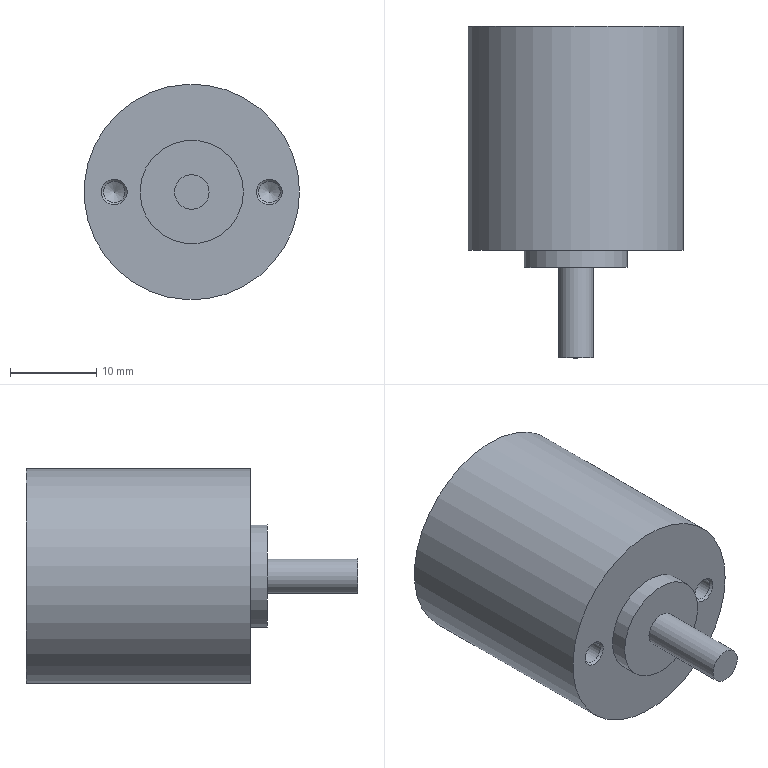Part | NX | features DATUM_CSYS 5, SKETCH 4, EXTRUDE 3, SIMPLE HOLE 2, SYMBOLIC_THREAD 2, HOLE PACKAGE 1 | 1 solid | 13 faces | box 25 x 38.5 x 25 mm | volume 13059 mm3 | cylinder 5 | plane 4 | cone 4 | commonest cylinder face diameters 2.5 x2 4 x1 12 x1 25 x1
STEP:
#1=CARTESIAN_POINT('',(12.5,-26.,0.));
#2=VERTEX_POINT('',#1);
#3=CARTESIAN_POINT('',(0.,-26.,0.));
#4=DIRECTION('',(0.,-1.,0.));
#5=DIRECTION('',(1.,0.,0.));
#6=AXIS2_PLACEMENT_3D('',#3,#4,#5);
#7=CIRCLE('',#6,12.5);
#8=EDGE_CURVE('',#2,#2,#7,.T.);
#9=ORIENTED_EDGE('',*,*,#8,.F.);
#10=EDGE_LOOP('',(#9));
#11=FACE_BOUND('',#10,.T.);
#12=CARTESIAN_POINT('',(12.5,0.,0.));
#13=VERTEX_POINT('',#12);
#14=CARTESIAN_POINT('',(0.,0.,0.));
#15=DIRECTION('',(0.,-1.,0.));
#16=DIRECTION('',(1.,0.,0.));
#17=AXIS2_PLACEMENT_3D('',#14,#15,#16);
#18=CIRCLE('',#17,12.5);
#19=EDGE_CURVE('',#13,#13,#18,.T.);
#20=ORIENTED_EDGE('',*,*,#19,.T.);
#21=EDGE_LOOP('',(#20));
#22=FACE_BOUND('',#21,.T.);
#23=CARTESIAN_POINT('',(0.,-26.,0.));
#24=DIRECTION('',(0.,1.,0.));
#25=DIRECTION('',(0.,0.,1.));
#26=AXIS2_PLACEMENT_3D('',#23,#24,#25);
#27=CYLINDRICAL_SURFACE('',#26,12.5);
#28=ADVANCED_FACE('',(#11,#22),#27,.T.);
#29=CARTESIAN_POINT('',(9.,-26.,-1.5));
#30=VERTEX_POINT('',#29);
#31=CARTESIAN_POINT('',(9.,-26.,0.));
#32=DIRECTION('',(0.,-1.,0.));
#33=DIRECTION('',(0.,0.,-1.));
#34=AXIS2_PLACEMENT_3D('',#31,#32,#33);
#35=CIRCLE('',#34,1.5);
#36=EDGE_CURVE('',#30,#30,#35,.F.);
#37=ORIENTED_EDGE('',*,*,#36,.T.);
#38=EDGE_LOOP('',(#37));
#39=FACE_BOUND('',#38,.T.);
#40=CARTESIAN_POINT('',(-9.,-26.,-1.5));
#41=VERTEX_POINT('',#40);
#42=CARTESIAN_POINT('',(-9.,-26.,0.));
#43=DIRECTION('',(0.,-1.,0.));
#44=DIRECTION('',(0.,0.,-1.));
#45=AXIS2_PLACEMENT_3D('',#42,#43,#44);
#46=CIRCLE('',#45,1.5);
#47=EDGE_CURVE('',#41,#41,#46,.F.);
#48=ORIENTED_EDGE('',*,*,#47,.T.);
#49=EDGE_LOOP('',(#48));
#50=FACE_BOUND('',#49,.T.);
#51=CARTESIAN_POINT('',(6.,-26.,0.));
#52=VERTEX_POINT('',#51);
#53=CARTESIAN_POINT('',(0.,-26.,0.));
#54=DIRECTION('',(0.,-1.,0.));
#55=DIRECTION('',(1.,0.,0.));
#56=AXIS2_PLACEMENT_3D('',#53,#54,#55);
#57=CIRCLE('',#56,6.);
#58=EDGE_CURVE('',#52,#52,#57,.T.);
#59=ORIENTED_EDGE('',*,*,#58,.F.);
#60=EDGE_LOOP('',(#59));
#61=FACE_BOUND('',#60,.T.);
#62=ORIENTED_EDGE('',*,*,#8,.T.);
#63=EDGE_LOOP('',(#62));
#64=FACE_BOUND('',#63,.T.);
#65=CARTESIAN_POINT('',(0.,-26.,0.));
#66=DIRECTION('',(0.,-1.,0.));
#67=DIRECTION('',(0.,0.,-1.));
#68=AXIS2_PLACEMENT_3D('',#65,#66,#67);
#69=PLANE('',#68);
#70=ADVANCED_FACE('',(#39,#50,#61,#64),#69,.T.);
#71=ORIENTED_EDGE('',*,*,#19,.F.);
#72=EDGE_LOOP('',(#71));
#73=FACE_BOUND('',#72,.T.);
#74=CARTESIAN_POINT('',(0.,0.,0.));
#75=DIRECTION('',(0.,-1.,0.));
#76=DIRECTION('',(0.,0.,-1.));
#77=AXIS2_PLACEMENT_3D('',#74,#75,#76);
#78=PLANE('',#77);
#79=ADVANCED_FACE('',(#73),#78,.F.);
#80=CARTESIAN_POINT('',(6.,-28.,0.));
#81=VERTEX_POINT('',#80);
#82=CARTESIAN_POINT('',(0.,-28.,0.));
#83=DIRECTION('',(0.,-1.,0.));
#84=DIRECTION('',(1.,0.,0.));
#85=AXIS2_PLACEMENT_3D('',#82,#83,#84);
#86=CIRCLE('',#85,6.);
#87=EDGE_CURVE('',#81,#81,#86,.T.);
#88=ORIENTED_EDGE('',*,*,#87,.F.);
#89=EDGE_LOOP('',(#88));
#90=FACE_BOUND('',#89,.T.);
#91=ORIENTED_EDGE('',*,*,#58,.T.);
#92=EDGE_LOOP('',(#91));
#93=FACE_BOUND('',#92,.T.);
#94=CARTESIAN_POINT('',(0.,-28.,0.));
#95=DIRECTION('',(0.,1.,0.));
#96=DIRECTION('',(0.,0.,1.));
#97=AXIS2_PLACEMENT_3D('',#94,#95,#96);
#98=CYLINDRICAL_SURFACE('',#97,6.);
#99=ADVANCED_FACE('',(#90,#93),#98,.T.);
#100=CARTESIAN_POINT('',(2.,-28.,0.));
#101=VERTEX_POINT('',#100);
#102=CARTESIAN_POINT('',(0.,-28.,0.));
#103=DIRECTION('',(0.,-1.,0.));
#104=DIRECTION('',(1.,0.,0.));
#105=AXIS2_PLACEMENT_3D('',#102,#103,#104);
#106=CIRCLE('',#105,2.);
#107=EDGE_CURVE('',#101,#101,#106,.T.);
#108=ORIENTED_EDGE('',*,*,#107,.F.);
#109=EDGE_LOOP('',(#108));
#110=FACE_BOUND('',#109,.T.);
#111=ORIENTED_EDGE('',*,*,#87,.T.);
#112=EDGE_LOOP('',(#111));
#113=FACE_BOUND('',#112,.T.);
#114=CARTESIAN_POINT('',(0.,-28.,0.));
#115=DIRECTION('',(0.,-1.,0.));
#116=DIRECTION('',(0.,0.,-1.));
#117=AXIS2_PLACEMENT_3D('',#114,#115,#116);
#118=PLANE('',#117);
#119=ADVANCED_FACE('',(#110,#113),#118,.T.);
#120=CARTESIAN_POINT('',(2.,-38.5,0.));
#121=VERTEX_POINT('',#120);
#122=CARTESIAN_POINT('',(0.,-38.5,0.));
#123=DIRECTION('',(0.,-1.,0.));
#124=DIRECTION('',(1.,0.,0.));
#125=AXIS2_PLACEMENT_3D('',#122,#123,#124);
#126=CIRCLE('',#125,2.);
#127=EDGE_CURVE('',#121,#121,#126,.T.);
#128=ORIENTED_EDGE('',*,*,#127,.F.);
#129=EDGE_LOOP('',(#128));
#130=FACE_BOUND('',#129,.T.);
#131=ORIENTED_EDGE('',*,*,#107,.T.);
#132=EDGE_LOOP('',(#131));
#133=FACE_BOUND('',#132,.T.);
#134=CARTESIAN_POINT('',(0.,-38.5,0.));
#135=DIRECTION('',(0.,1.,0.));
#136=DIRECTION('',(0.,0.,1.));
#137=AXIS2_PLACEMENT_3D('',#134,#135,#136);
#138=CYLINDRICAL_SURFACE('',#137,2.);
#139=ADVANCED_FACE('',(#130,#133),#138,.T.);
#140=ORIENTED_EDGE('',*,*,#127,.T.);
#141=EDGE_LOOP('',(#140));
#142=FACE_BOUND('',#141,.T.);
#143=CARTESIAN_POINT('',(0.,-38.5,0.));
#144=DIRECTION('',(0.,-1.,0.));
#145=DIRECTION('',(0.,0.,-1.));
#146=AXIS2_PLACEMENT_3D('',#143,#144,#145);
#147=PLANE('',#146);
#148=ADVANCED_FACE('',(#142),#147,.T.);
#149=CARTESIAN_POINT('',(-9.,-20.,1.25));
#150=VERTEX_POINT('',#149);
#151=CARTESIAN_POINT('',(-9.,-20.,0.));
#152=DIRECTION('',(0.,1.,0.));
#153=DIRECTION('',(0.,0.,1.));
#154=AXIS2_PLACEMENT_3D('',#151,#152,#153);
#155=CIRCLE('',#154,1.25);
#156=EDGE_CURVE('',#150,#150,#155,.F.);
#157=ORIENTED_EDGE('',*,*,#156,.T.);
#158=EDGE_LOOP('',(#157));
#159=FACE_BOUND('',#158,.T.);
#160=CARTESIAN_POINT('',(-9.,-19.249,0.));
#161=VERTEX_POINT('',#160);
#162=VERTEX_LOOP('',#161);
#163=FACE_BOUND('',#162,.T.);
#164=CARTESIAN_POINT('',(-9.,-20.,0.));
#165=DIRECTION('',(0.,-1.,0.));
#166=DIRECTION('',(0.,0.,-1.));
#167=AXIS2_PLACEMENT_3D('',#164,#165,#166);
#168=CONICAL_SURFACE('',#167,1.25,1.03);
#169=ADVANCED_FACE('',(#159,#163),#168,.F.);
#170=CARTESIAN_POINT('',(-9.,-25.75,-1.25));
#171=VERTEX_POINT('',#170);
#172=CARTESIAN_POINT('',(-9.,-25.75,0.));
#173=DIRECTION('',(0.,-1.,0.));
#174=DIRECTION('',(0.,0.,-1.));
#175=AXIS2_PLACEMENT_3D('',#172,#173,#174);
#176=CIRCLE('',#175,1.25);
#177=EDGE_CURVE('',#171,#171,#176,.T.);
#178=ORIENTED_EDGE('',*,*,#177,.T.);
#179=EDGE_LOOP('',(#178));
#180=FACE_BOUND('',#179,.T.);
#181=ORIENTED_EDGE('',*,*,#156,.F.);
#182=EDGE_LOOP('',(#181));
#183=FACE_BOUND('',#182,.T.);
#184=CARTESIAN_POINT('',(-9.,-26.,0.));
#185=DIRECTION('',(0.,1.,0.));
#186=DIRECTION('',(0.,0.,1.));
#187=AXIS2_PLACEMENT_3D('',#184,#185,#186);
#188=CYLINDRICAL_SURFACE('',#187,1.25);
#189=ADVANCED_FACE('',(#180,#183),#188,.F.);
#190=ORIENTED_EDGE('',*,*,#177,.F.);
#191=EDGE_LOOP('',(#190));
#192=FACE_BOUND('',#191,.T.);
#193=ORIENTED_EDGE('',*,*,#47,.F.);
#194=EDGE_LOOP('',(#193));
#195=FACE_BOUND('',#194,.T.);
#196=CARTESIAN_POINT('',(-9.,-26.,0.));
#197=DIRECTION('',(0.,-1.,0.));
#198=DIRECTION('',(0.,0.,-1.));
#199=AXIS2_PLACEMENT_3D('',#196,#197,#198);
#200=CONICAL_SURFACE('',#199,1.5,0.7854);
#201=ADVANCED_FACE('',(#192,#195),#200,.F.);
#202=CARTESIAN_POINT('',(9.,-20.,1.25));
#203=VERTEX_POINT('',#202);
#204=CARTESIAN_POINT('',(9.,-20.,0.));
#205=DIRECTION('',(0.,1.,0.));
#206=DIRECTION('',(0.,0.,1.));
#207=AXIS2_PLACEMENT_3D('',#204,#205,#206);
#208=CIRCLE('',#207,1.25);
#209=EDGE_CURVE('',#203,#203,#208,.F.);
#210=ORIENTED_EDGE('',*,*,#209,.T.);
#211=EDGE_LOOP('',(#210));
#212=FACE_BOUND('',#211,.T.);
#213=CARTESIAN_POINT('',(9.,-19.249,0.));
#214=VERTEX_POINT('',#213);
#215=VERTEX_LOOP('',#214);
#216=FACE_BOUND('',#215,.T.);
#217=CARTESIAN_POINT('',(9.,-20.,0.));
#218=DIRECTION('',(0.,-1.,0.));
#219=DIRECTION('',(0.,0.,-1.));
#220=AXIS2_PLACEMENT_3D('',#217,#218,#219);
#221=CONICAL_SURFACE('',#220,1.25,1.03);
#222=ADVANCED_FACE('',(#212,#216),#221,.F.);
#223=CARTESIAN_POINT('',(9.,-25.75,-1.25));
#224=VERTEX_POINT('',#223);
#225=CARTESIAN_POINT('',(9.,-25.75,0.));
#226=DIRECTION('',(0.,-1.,0.));
#227=DIRECTION('',(0.,0.,-1.));
#228=AXIS2_PLACEMENT_3D('',#225,#226,#227);
#229=CIRCLE('',#228,1.25);
#230=EDGE_CURVE('',#224,#224,#229,.T.);
#231=ORIENTED_EDGE('',*,*,#230,.T.);
#232=EDGE_LOOP('',(#231));
#233=FACE_BOUND('',#232,.T.);
#234=ORIENTED_EDGE('',*,*,#209,.F.);
#235=EDGE_LOOP('',(#234));
#236=FACE_BOUND('',#235,.T.);
#237=CARTESIAN_POINT('',(9.,-26.,0.));
#238=DIRECTION('',(0.,1.,0.));
#239=DIRECTION('',(0.,0.,1.));
#240=AXIS2_PLACEMENT_3D('',#237,#238,#239);
#241=CYLINDRICAL_SURFACE('',#240,1.25);
#242=ADVANCED_FACE('',(#233,#236),#241,.F.);
#243=ORIENTED_EDGE('',*,*,#230,.F.);
#244=EDGE_LOOP('',(#243));
#245=FACE_BOUND('',#244,.T.);
#246=ORIENTED_EDGE('',*,*,#36,.F.);
#247=EDGE_LOOP('',(#246));
#248=FACE_BOUND('',#247,.T.);
#249=CARTESIAN_POINT('',(9.,-26.,0.));
#250=DIRECTION('',(0.,-1.,0.));
#251=DIRECTION('',(0.,0.,-1.));
#252=AXIS2_PLACEMENT_3D('',#249,#250,#251);
#253=CONICAL_SURFACE('',#252,1.5,0.7854);
#254=ADVANCED_FACE('',(#245,#248),#253,.F.);
#255=CLOSED_SHELL('',(#28,#70,#79,#99,#119,#139,#148,#169,#189,#201,#222,#242,#254));
#256=MANIFOLD_SOLID_BREP('',#255);
#257=(LENGTH_UNIT()NAMED_UNIT(*)SI_UNIT(.MILLI.,.METRE.));
#258=UNCERTAINTY_MEASURE_WITH_UNIT(LENGTH_MEASURE(0.00001),#257,'','');
#259=(NAMED_UNIT(*)PLANE_ANGLE_UNIT()SI_UNIT($,.RADIAN.));
#260=(NAMED_UNIT(*)SI_UNIT($,.STERADIAN.)SOLID_ANGLE_UNIT());
#261=(GEOMETRIC_REPRESENTATION_CONTEXT(3)GLOBAL_UNCERTAINTY_ASSIGNED_CONTEXT((#258))GLOBAL_UNIT_ASSIGNED_CONTEXT((#257,#259,#260))REPRESENTATION_CONTEXT('',''));
#262=ADVANCED_BREP_SHAPE_REPRESENTATION('',(#256),#261);